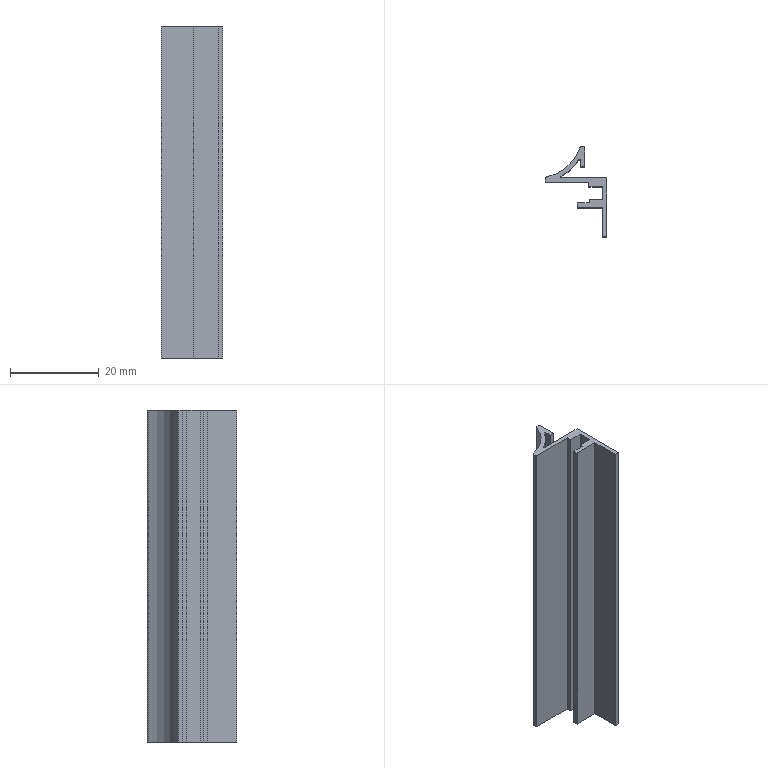Part | SolidWorks | features BaseBody 1, ICE 1, MoveFace 1 | 1 solid | 27 faces | box 14 x 20.3 x 75 mm | volume 3819 mm3 | plane 20 | cylinder 7 | commonest cylinder face diameters 0.387 x2 0.8 x2 0.4 x1 20 x1 22 x1
STEP:
#1=CARTESIAN_POINT('',(-5.304,-0.625,200.));
#2=VERTEX_POINT('',#1);
#3=CARTESIAN_POINT('',(-5.449,-0.8125,200.));
#4=VERTEX_POINT('',#3);
#5=CARTESIAN_POINT('',(-5.255,-0.8125,200.));
#6=DIRECTION('',(0.,0.,1.));
#7=DIRECTION('',(-1.,0.,0.));
#8=AXIS2_PLACEMENT_3D('',#5,#6,#7);
#9=CIRCLE('',#8,0.1937);
#10=EDGE_CURVE('',#2,#4,#9,.T.);
#11=ORIENTED_EDGE('',*,*,#10,.T.);
#12=CARTESIAN_POINT('',(-5.449,-0.8125,125.));
#13=VERTEX_POINT('',#12);
#14=CARTESIAN_POINT('',(-5.449,-0.8125,230.));
#15=DIRECTION('',(0.,0.,-1.));
#16=VECTOR('',#15,1000.);
#17=LINE('',#14,#16);
#18=EDGE_CURVE('',#4,#13,#17,.T.);
#19=ORIENTED_EDGE('',*,*,#18,.T.);
#20=CARTESIAN_POINT('',(-5.304,-0.625,125.));
#21=VERTEX_POINT('',#20);
#22=CARTESIAN_POINT('',(-5.255,-0.8125,125.));
#23=DIRECTION('',(0.,0.,-1.));
#24=DIRECTION('',(1.,0.,0.));
#25=AXIS2_PLACEMENT_3D('',#22,#23,#24);
#26=CIRCLE('',#25,0.1937);
#27=EDGE_CURVE('',#13,#21,#26,.T.);
#28=ORIENTED_EDGE('',*,*,#27,.T.);
#29=CARTESIAN_POINT('',(-5.304,-0.625,230.));
#30=DIRECTION('',(0.,0.,-1.));
#31=VECTOR('',#30,1000.);
#32=LINE('',#29,#31);
#33=EDGE_CURVE('',#2,#21,#32,.T.);
#34=ORIENTED_EDGE('',*,*,#33,.F.);
#35=EDGE_LOOP('',(#11,#19,#28,#34));
#36=FACE_OUTER_BOUND('',#35,.T.);
#37=CARTESIAN_POINT('',(-5.255,-0.8125,230.));
#38=DIRECTION('',(0.,0.,-1.));
#39=DIRECTION('',(-1.,0.,0.));
#40=AXIS2_PLACEMENT_3D('',#37,#38,#39);
#41=CYLINDRICAL_SURFACE('',#40,0.1937);
#42=ADVANCED_FACE('',(#36),#41,.F.);
#43=CARTESIAN_POINT('',(5.,-1.,125.));
#44=VERTEX_POINT('',#43);
#45=CARTESIAN_POINT('',(5.,-14.3,125.));
#46=VERTEX_POINT('',#45);
#47=CARTESIAN_POINT('',(5.,29.623,125.));
#48=DIRECTION('',(0.,-1.,0.));
#49=VECTOR('',#48,1000.);
#50=LINE('',#47,#49);
#51=EDGE_CURVE('',#44,#46,#50,.T.);
#52=ORIENTED_EDGE('',*,*,#51,.F.);
#53=CARTESIAN_POINT('',(5.,-1.,200.));
#54=VERTEX_POINT('',#53);
#55=CARTESIAN_POINT('',(5.,-1.,230.));
#56=DIRECTION('',(0.,0.,-1.));
#57=VECTOR('',#56,1000.);
#58=LINE('',#55,#57);
#59=EDGE_CURVE('',#54,#44,#58,.T.);
#60=ORIENTED_EDGE('',*,*,#59,.F.);
#61=CARTESIAN_POINT('',(5.,-14.3,200.));
#62=VERTEX_POINT('',#61);
#63=CARTESIAN_POINT('',(5.,-14.3,200.));
#64=DIRECTION('',(0.,1.,0.));
#65=VECTOR('',#64,1000.);
#66=LINE('',#63,#65);
#67=EDGE_CURVE('',#62,#54,#66,.T.);
#68=ORIENTED_EDGE('',*,*,#67,.F.);
#69=CARTESIAN_POINT('',(5.,-14.3,230.));
#70=DIRECTION('',(0.,0.,1.));
#71=VECTOR('',#70,1000.);
#72=LINE('',#69,#71);
#73=EDGE_CURVE('',#46,#62,#72,.T.);
#74=ORIENTED_EDGE('',*,*,#73,.F.);
#75=EDGE_LOOP('',(#52,#60,#68,#74));
#76=FACE_OUTER_BOUND('',#75,.T.);
#77=CARTESIAN_POINT('',(5.,-14.3,230.));
#78=DIRECTION('',(-1.,0.,0.));
#79=DIRECTION('',(0.,0.,1.));
#80=AXIS2_PLACEMENT_3D('',#77,#78,#79);
#81=PLANE('',#80);
#82=ADVANCED_FACE('',(#76),#81,.F.);
#83=CARTESIAN_POINT('',(-9.,-2.,125.));
#84=VERTEX_POINT('',#83);
#85=CARTESIAN_POINT('',(-9.,-2.,200.));
#86=VERTEX_POINT('',#85);
#87=CARTESIAN_POINT('',(-9.,-2.,230.));
#88=DIRECTION('',(0.,0.,1.));
#89=VECTOR('',#88,1000.);
#90=LINE('',#87,#89);
#91=EDGE_CURVE('',#84,#86,#90,.T.);
#92=ORIENTED_EDGE('',*,*,#91,.F.);
#93=CARTESIAN_POINT('',(0.9,-2.,125.));
#94=VERTEX_POINT('',#93);
#95=CARTESIAN_POINT('',(5.,-2.,125.));
#96=DIRECTION('',(-1.,0.,0.));
#97=VECTOR('',#96,1000.);
#98=LINE('',#95,#97);
#99=EDGE_CURVE('',#94,#84,#98,.T.);
#100=ORIENTED_EDGE('',*,*,#99,.F.);
#101=CARTESIAN_POINT('',(0.9,-2.,200.));
#102=VERTEX_POINT('',#101);
#103=CARTESIAN_POINT('',(0.9,-2.,230.));
#104=DIRECTION('',(0.,0.,-1.));
#105=VECTOR('',#104,1000.);
#106=LINE('',#103,#105);
#107=EDGE_CURVE('',#102,#94,#106,.T.);
#108=ORIENTED_EDGE('',*,*,#107,.F.);
#109=CARTESIAN_POINT('',(5.,-2.,200.));
#110=DIRECTION('',(1.,0.,0.));
#111=VECTOR('',#110,1000.);
#112=LINE('',#109,#111);
#113=EDGE_CURVE('',#86,#102,#112,.T.);
#114=ORIENTED_EDGE('',*,*,#113,.F.);
#115=EDGE_LOOP('',(#92,#100,#108,#114));
#116=FACE_OUTER_BOUND('',#115,.T.);
#117=CARTESIAN_POINT('',(-9.,-2.,230.));
#118=DIRECTION('',(0.,1.,0.));
#119=DIRECTION('',(0.,0.,1.));
#120=AXIS2_PLACEMENT_3D('',#117,#118,#119);
#121=PLANE('',#120);
#122=ADVANCED_FACE('',(#116),#121,.F.);
#123=CARTESIAN_POINT('',(4.,-6.,200.));
#124=VERTEX_POINT('',#123);
#125=CARTESIAN_POINT('',(4.,-3.,200.));
#126=VERTEX_POINT('',#125);
#127=CARTESIAN_POINT('',(4.,29.623,200.));
#128=DIRECTION('',(0.,1.,0.));
#129=VECTOR('',#128,1000.);
#130=LINE('',#127,#129);
#131=EDGE_CURVE('',#124,#126,#130,.T.);
#132=ORIENTED_EDGE('',*,*,#131,.F.);
#133=CARTESIAN_POINT('',(1.,-6.,200.));
#134=VERTEX_POINT('',#133);
#135=CARTESIAN_POINT('',(5.,-6.,200.));
#136=DIRECTION('',(1.,0.,0.));
#137=VECTOR('',#136,1000.);
#138=LINE('',#135,#137);
#139=EDGE_CURVE('',#134,#124,#138,.T.);
#140=ORIENTED_EDGE('',*,*,#139,.F.);
#141=CARTESIAN_POINT('',(1.,-6.7,200.));
#142=VERTEX_POINT('',#141);
#143=CARTESIAN_POINT('',(1.,-6.,200.));
#144=DIRECTION('',(0.,-1.,0.));
#145=VECTOR('',#144,1000.);
#146=LINE('',#143,#145);
#147=EDGE_CURVE('',#134,#142,#146,.T.);
#148=ORIENTED_EDGE('',*,*,#147,.T.);
#149=CARTESIAN_POINT('',(-1.7,-6.7,200.));
#150=VERTEX_POINT('',#149);
#151=CARTESIAN_POINT('',(5.,-6.7,200.));
#152=DIRECTION('',(1.,0.,0.));
#153=VECTOR('',#152,1000.);
#154=LINE('',#151,#153);
#155=EDGE_CURVE('',#150,#142,#154,.T.);
#156=ORIENTED_EDGE('',*,*,#155,.F.);
#157=CARTESIAN_POINT('',(-1.7,-7.7,200.));
#158=VERTEX_POINT('',#157);
#159=CARTESIAN_POINT('',(-1.7,-6.7,200.));
#160=DIRECTION('',(0.,-1.,0.));
#161=VECTOR('',#160,1000.);
#162=LINE('',#159,#161);
#163=EDGE_CURVE('',#150,#158,#162,.T.);
#164=ORIENTED_EDGE('',*,*,#163,.T.);
#165=CARTESIAN_POINT('',(4.,-7.7,200.));
#166=VERTEX_POINT('',#165);
#167=CARTESIAN_POINT('',(5.,-7.7,200.));
#168=DIRECTION('',(-1.,0.,0.));
#169=VECTOR('',#168,1000.);
#170=LINE('',#167,#169);
#171=EDGE_CURVE('',#166,#158,#170,.T.);
#172=ORIENTED_EDGE('',*,*,#171,.F.);
#173=CARTESIAN_POINT('',(4.,-14.3,200.));
#174=VERTEX_POINT('',#173);
#175=CARTESIAN_POINT('',(4.,29.623,200.));
#176=DIRECTION('',(0.,1.,0.));
#177=VECTOR('',#176,1000.);
#178=LINE('',#175,#177);
#179=EDGE_CURVE('',#174,#166,#178,.T.);
#180=ORIENTED_EDGE('',*,*,#179,.F.);
#181=CARTESIAN_POINT('',(5.,-14.3,200.));
#182=DIRECTION('',(-1.,0.,0.));
#183=VECTOR('',#182,1000.);
#184=LINE('',#181,#183);
#185=EDGE_CURVE('',#62,#174,#184,.T.);
#186=ORIENTED_EDGE('',*,*,#185,.F.);
#187=ORIENTED_EDGE('',*,*,#67,.T.);
#188=CARTESIAN_POINT('',(-5.207,-1.,200.));
#189=VERTEX_POINT('',#188);
#190=CARTESIAN_POINT('',(5.,-1.,200.));
#191=DIRECTION('',(1.,0.,0.));
#192=VECTOR('',#191,1000.);
#193=LINE('',#190,#192);
#194=EDGE_CURVE('',#189,#54,#193,.T.);
#195=ORIENTED_EDGE('',*,*,#194,.F.);
#196=CARTESIAN_POINT('',(-5.255,-0.8125,200.));
#197=DIRECTION('',(0.,0.,1.));
#198=DIRECTION('',(-1.,0.,0.));
#199=AXIS2_PLACEMENT_3D('',#196,#197,#198);
#200=CIRCLE('',#199,0.1937);
#201=EDGE_CURVE('',#4,#189,#200,.T.);
#202=ORIENTED_EDGE('',*,*,#201,.F.);
#203=ORIENTED_EDGE('',*,*,#10,.F.);
#204=CARTESIAN_POINT('',(-1.368,3.063,200.));
#205=VERTEX_POINT('',#204);
#206=CARTESIAN_POINT('',(-10.628,9.,200.));
#207=DIRECTION('',(0.,0.,1.));
#208=DIRECTION('',(-1.,0.,0.));
#209=AXIS2_PLACEMENT_3D('',#206,#207,#208);
#210=CIRCLE('',#209,11.);
#211=EDGE_CURVE('',#2,#205,#210,.T.);
#212=ORIENTED_EDGE('',*,*,#211,.T.);
#213=CARTESIAN_POINT('',(-1.,2.955,200.));
#214=VERTEX_POINT('',#213);
#215=CARTESIAN_POINT('',(-1.2,2.955,200.));
#216=DIRECTION('',(0.,0.,1.));
#217=DIRECTION('',(-1.,0.,0.));
#218=AXIS2_PLACEMENT_3D('',#215,#216,#217);
#219=CIRCLE('',#218,0.2);
#220=EDGE_CURVE('',#214,#205,#219,.T.);
#221=ORIENTED_EDGE('',*,*,#220,.F.);
#222=CARTESIAN_POINT('',(-1.,1.5,200.));
#223=VERTEX_POINT('',#222);
#224=CARTESIAN_POINT('',(-1.,2.955,200.));
#225=DIRECTION('',(0.,1.,0.));
#226=VECTOR('',#225,1000.);
#227=LINE('',#224,#226);
#228=EDGE_CURVE('',#223,#214,#227,.T.);
#229=ORIENTED_EDGE('',*,*,#228,.F.);
#230=CARTESIAN_POINT('',(0.,1.5,200.));
#231=VERTEX_POINT('',#230);
#232=CARTESIAN_POINT('',(-1.,1.5,200.));
#233=DIRECTION('',(-1.,0.,0.));
#234=VECTOR('',#233,1000.);
#235=LINE('',#232,#234);
#236=EDGE_CURVE('',#231,#223,#235,.T.);
#237=ORIENTED_EDGE('',*,*,#236,.F.);
#238=CARTESIAN_POINT('',(0.,6.,200.));
#239=VERTEX_POINT('',#238);
#240=CARTESIAN_POINT('',(0.,1.5,200.));
#241=DIRECTION('',(0.,-1.,0.));
#242=VECTOR('',#241,1000.);
#243=LINE('',#240,#242);
#244=EDGE_CURVE('',#239,#231,#243,.T.);
#245=ORIENTED_EDGE('',*,*,#244,.F.);
#246=CARTESIAN_POINT('',(-0.8,6.,200.));
#247=VERTEX_POINT('',#246);
#248=CARTESIAN_POINT('',(0.,6.,200.));
#249=DIRECTION('',(1.,0.,0.));
#250=VECTOR('',#249,1000.);
#251=LINE('',#248,#250);
#252=EDGE_CURVE('',#247,#239,#251,.T.);
#253=ORIENTED_EDGE('',*,*,#252,.F.);
#254=CARTESIAN_POINT('',(-1.178,5.731,200.));
#255=VERTEX_POINT('',#254);
#256=CARTESIAN_POINT('',(-0.8,5.6,200.));
#257=DIRECTION('',(0.,0.,1.));
#258=DIRECTION('',(-1.,0.,0.));
#259=AXIS2_PLACEMENT_3D('',#256,#257,#258);
#260=CIRCLE('',#259,0.4);
#261=EDGE_CURVE('',#247,#255,#260,.T.);
#262=ORIENTED_EDGE('',*,*,#261,.T.);
#263=CARTESIAN_POINT('',(-8.678,-0.8077,200.));
#264=VERTEX_POINT('',#263);
#265=CARTESIAN_POINT('',(-10.628,9.,200.));
#266=DIRECTION('',(0.,0.,1.));
#267=DIRECTION('',(-1.,0.,0.));
#268=AXIS2_PLACEMENT_3D('',#265,#266,#267);
#269=CIRCLE('',#268,10.);
#270=EDGE_CURVE('',#264,#255,#269,.T.);
#271=ORIENTED_EDGE('',*,*,#270,.F.);
#272=CARTESIAN_POINT('',(-9.,-1.2,200.));
#273=VERTEX_POINT('',#272);
#274=CARTESIAN_POINT('',(-8.6,-1.2,200.));
#275=DIRECTION('',(0.,0.,1.));
#276=DIRECTION('',(-1.,0.,0.));
#277=AXIS2_PLACEMENT_3D('',#274,#275,#276);
#278=CIRCLE('',#277,0.4);
#279=EDGE_CURVE('',#264,#273,#278,.T.);
#280=ORIENTED_EDGE('',*,*,#279,.T.);
#281=CARTESIAN_POINT('',(-9.,8.,200.));
#282=DIRECTION('',(0.,-1.,0.));
#283=VECTOR('',#282,1000.);
#284=LINE('',#281,#283);
#285=EDGE_CURVE('',#273,#86,#284,.T.);
#286=ORIENTED_EDGE('',*,*,#285,.T.);
#287=ORIENTED_EDGE('',*,*,#113,.T.);
#288=CARTESIAN_POINT('',(0.9,-3.,200.));
#289=VERTEX_POINT('',#288);
#290=CARTESIAN_POINT('',(0.9,29.623,200.));
#291=DIRECTION('',(0.,1.,0.));
#292=VECTOR('',#291,1000.);
#293=LINE('',#290,#292);
#294=EDGE_CURVE('',#289,#102,#293,.T.);
#295=ORIENTED_EDGE('',*,*,#294,.F.);
#296=CARTESIAN_POINT('',(5.,-3.,200.));
#297=DIRECTION('',(-1.,0.,0.));
#298=VECTOR('',#297,1000.);
#299=LINE('',#296,#298);
#300=EDGE_CURVE('',#126,#289,#299,.T.);
#301=ORIENTED_EDGE('',*,*,#300,.F.);
#302=EDGE_LOOP('',(#132,#140,#148,#156,#164,#172,#180,#186,#187,#195,#202,#203,#212,#221,#229,#237,#245,#253,#262,#271,#280,#286,#287,#295,#301));
#303=FACE_OUTER_BOUND('',#302,.T.);
#304=CARTESIAN_POINT('',(5.,29.623,200.));
#305=DIRECTION('',(0.,0.,-1.));
#306=DIRECTION('',(-1.,0.,0.));
#307=AXIS2_PLACEMENT_3D('',#304,#305,#306);
#308=PLANE('',#307);
#309=ADVANCED_FACE('',(#303),#308,.F.);
#310=ORIENTED_EDGE('',*,*,#185,.T.);
#311=CARTESIAN_POINT('',(4.,-14.3,125.));
#312=VERTEX_POINT('',#311);
#313=CARTESIAN_POINT('',(4.,-14.3,230.));
#314=DIRECTION('',(0.,0.,1.));
#315=VECTOR('',#314,1000.);
#316=LINE('',#313,#315);
#317=EDGE_CURVE('',#312,#174,#316,.T.);
#318=ORIENTED_EDGE('',*,*,#317,.F.);
#319=CARTESIAN_POINT('',(5.,-14.3,125.));
#320=DIRECTION('',(-1.,0.,0.));
#321=VECTOR('',#320,1000.);
#322=LINE('',#319,#321);
#323=EDGE_CURVE('',#46,#312,#322,.T.);
#324=ORIENTED_EDGE('',*,*,#323,.F.);
#325=ORIENTED_EDGE('',*,*,#73,.T.);
#326=EDGE_LOOP('',(#310,#318,#324,#325));
#327=FACE_OUTER_BOUND('',#326,.T.);
#328=CARTESIAN_POINT('',(4.,-14.3,230.));
#329=DIRECTION('',(0.,1.,0.));
#330=DIRECTION('',(0.,0.,1.));
#331=AXIS2_PLACEMENT_3D('',#328,#329,#330);
#332=PLANE('',#331);
#333=ADVANCED_FACE('',(#327),#332,.F.);
#334=ORIENTED_EDGE('',*,*,#51,.T.);
#335=ORIENTED_EDGE('',*,*,#323,.T.);
#336=CARTESIAN_POINT('',(4.,-7.7,125.));
#337=VERTEX_POINT('',#336);
#338=CARTESIAN_POINT('',(4.,-7.7,125.));
#339=DIRECTION('',(0.,-1.,0.));
#340=VECTOR('',#339,1000.);
#341=LINE('',#338,#340);
#342=EDGE_CURVE('',#337,#312,#341,.T.);
#343=ORIENTED_EDGE('',*,*,#342,.F.);
#344=CARTESIAN_POINT('',(-1.7,-7.7,125.));
#345=VERTEX_POINT('',#344);
#346=CARTESIAN_POINT('',(-1.7,-7.7,125.));
#347=DIRECTION('',(1.,0.,0.));
#348=VECTOR('',#347,1000.);
#349=LINE('',#346,#348);
#350=EDGE_CURVE('',#345,#337,#349,.T.);
#351=ORIENTED_EDGE('',*,*,#350,.F.);
#352=CARTESIAN_POINT('',(-1.7,-6.7,125.));
#353=VERTEX_POINT('',#352);
#354=CARTESIAN_POINT('',(-1.7,29.623,125.));
#355=DIRECTION('',(0.,1.,0.));
#356=VECTOR('',#355,1000.);
#357=LINE('',#354,#356);
#358=EDGE_CURVE('',#345,#353,#357,.T.);
#359=ORIENTED_EDGE('',*,*,#358,.T.);
#360=CARTESIAN_POINT('',(1.,-6.7,125.));
#361=VERTEX_POINT('',#360);
#362=CARTESIAN_POINT('',(1.,-6.7,125.));
#363=DIRECTION('',(-1.,0.,0.));
#364=VECTOR('',#363,1000.);
#365=LINE('',#362,#364);
#366=EDGE_CURVE('',#361,#353,#365,.T.);
#367=ORIENTED_EDGE('',*,*,#366,.F.);
#368=CARTESIAN_POINT('',(1.,-6.,125.));
#369=VERTEX_POINT('',#368);
#370=CARTESIAN_POINT('',(1.,29.623,125.));
#371=DIRECTION('',(0.,1.,0.));
#372=VECTOR('',#371,1000.);
#373=LINE('',#370,#372);
#374=EDGE_CURVE('',#361,#369,#373,.T.);
#375=ORIENTED_EDGE('',*,*,#374,.T.);
#376=CARTESIAN_POINT('',(4.,-6.,125.));
#377=VERTEX_POINT('',#376);
#378=CARTESIAN_POINT('',(4.,-6.,125.));
#379=DIRECTION('',(-1.,0.,0.));
#380=VECTOR('',#379,1000.);
#381=LINE('',#378,#380);
#382=EDGE_CURVE('',#377,#369,#381,.T.);
#383=ORIENTED_EDGE('',*,*,#382,.F.);
#384=CARTESIAN_POINT('',(4.,-3.,125.));
#385=VERTEX_POINT('',#384);
#386=CARTESIAN_POINT('',(4.,-3.,125.));
#387=DIRECTION('',(0.,-1.,0.));
#388=VECTOR('',#387,1000.);
#389=LINE('',#386,#388);
#390=EDGE_CURVE('',#385,#377,#389,.T.);
#391=ORIENTED_EDGE('',*,*,#390,.F.);
#392=CARTESIAN_POINT('',(0.9,-3.,125.));
#393=VERTEX_POINT('',#392);
#394=CARTESIAN_POINT('',(0.9,-3.,125.));
#395=DIRECTION('',(1.,0.,0.));
#396=VECTOR('',#395,1000.);
#397=LINE('',#394,#396);
#398=EDGE_CURVE('',#393,#385,#397,.T.);
#399=ORIENTED_EDGE('',*,*,#398,.F.);
#400=CARTESIAN_POINT('',(0.9,-2.,125.));
#401=DIRECTION('',(0.,-1.,0.));
#402=VECTOR('',#401,1000.);
#403=LINE('',#400,#402);
#404=EDGE_CURVE('',#94,#393,#403,.T.);
#405=ORIENTED_EDGE('',*,*,#404,.F.);
#406=ORIENTED_EDGE('',*,*,#99,.T.);
#407=CARTESIAN_POINT('',(-9.,-1.2,125.));
#408=VERTEX_POINT('',#407);
#409=CARTESIAN_POINT('',(-9.,-1.2,125.));
#410=DIRECTION('',(0.,-1.,0.));
#411=VECTOR('',#410,1000.);
#412=LINE('',#409,#411);
#413=EDGE_CURVE('',#408,#84,#412,.T.);
#414=ORIENTED_EDGE('',*,*,#413,.F.);
#415=CARTESIAN_POINT('',(-8.678,-0.8077,125.));
#416=VERTEX_POINT('',#415);
#417=CARTESIAN_POINT('',(-8.6,-1.2,125.));
#418=DIRECTION('',(0.,0.,-1.));
#419=DIRECTION('',(1.,0.,0.));
#420=AXIS2_PLACEMENT_3D('',#417,#418,#419);
#421=CIRCLE('',#420,0.4);
#422=EDGE_CURVE('',#408,#416,#421,.T.);
#423=ORIENTED_EDGE('',*,*,#422,.T.);
#424=CARTESIAN_POINT('',(-1.178,5.731,125.));
#425=VERTEX_POINT('',#424);
#426=CARTESIAN_POINT('',(-10.628,9.,125.));
#427=DIRECTION('',(0.,0.,-1.));
#428=DIRECTION('',(1.,0.,0.));
#429=AXIS2_PLACEMENT_3D('',#426,#427,#428);
#430=CIRCLE('',#429,10.);
#431=EDGE_CURVE('',#425,#416,#430,.T.);
#432=ORIENTED_EDGE('',*,*,#431,.F.);
#433=CARTESIAN_POINT('',(-0.8,6.,125.));
#434=VERTEX_POINT('',#433);
#435=CARTESIAN_POINT('',(-0.8,5.6,125.));
#436=DIRECTION('',(0.,0.,-1.));
#437=DIRECTION('',(1.,0.,0.));
#438=AXIS2_PLACEMENT_3D('',#435,#436,#437);
#439=CIRCLE('',#438,0.4);
#440=EDGE_CURVE('',#425,#434,#439,.T.);
#441=ORIENTED_EDGE('',*,*,#440,.T.);
#442=CARTESIAN_POINT('',(0.,6.,125.));
#443=VERTEX_POINT('',#442);
#444=CARTESIAN_POINT('',(0.,6.,125.));
#445=DIRECTION('',(-1.,0.,0.));
#446=VECTOR('',#445,1000.);
#447=LINE('',#444,#446);
#448=EDGE_CURVE('',#443,#434,#447,.T.);
#449=ORIENTED_EDGE('',*,*,#448,.F.);
#450=CARTESIAN_POINT('',(0.,1.5,125.));
#451=VERTEX_POINT('',#450);
#452=CARTESIAN_POINT('',(0.,1.5,125.));
#453=DIRECTION('',(0.,1.,0.));
#454=VECTOR('',#453,1000.);
#455=LINE('',#452,#454);
#456=EDGE_CURVE('',#451,#443,#455,.T.);
#457=ORIENTED_EDGE('',*,*,#456,.F.);
#458=CARTESIAN_POINT('',(-1.,1.5,125.));
#459=VERTEX_POINT('',#458);
#460=CARTESIAN_POINT('',(-1.,1.5,125.));
#461=DIRECTION('',(1.,0.,0.));
#462=VECTOR('',#461,1000.);
#463=LINE('',#460,#462);
#464=EDGE_CURVE('',#459,#451,#463,.T.);
#465=ORIENTED_EDGE('',*,*,#464,.F.);
#466=CARTESIAN_POINT('',(-1.,2.955,125.));
#467=VERTEX_POINT('',#466);
#468=CARTESIAN_POINT('',(-1.,2.955,125.));
#469=DIRECTION('',(0.,-1.,0.));
#470=VECTOR('',#469,1000.);
#471=LINE('',#468,#470);
#472=EDGE_CURVE('',#467,#459,#471,.T.);
#473=ORIENTED_EDGE('',*,*,#472,.F.);
#474=CARTESIAN_POINT('',(-1.368,3.063,125.));
#475=VERTEX_POINT('',#474);
#476=CARTESIAN_POINT('',(-1.2,2.955,125.));
#477=DIRECTION('',(0.,0.,-1.));
#478=DIRECTION('',(1.,0.,0.));
#479=AXIS2_PLACEMENT_3D('',#476,#477,#478);
#480=CIRCLE('',#479,0.2);
#481=EDGE_CURVE('',#475,#467,#480,.T.);
#482=ORIENTED_EDGE('',*,*,#481,.F.);
#483=CARTESIAN_POINT('',(-10.628,9.,125.));
#484=DIRECTION('',(0.,0.,-1.));
#485=DIRECTION('',(1.,0.,0.));
#486=AXIS2_PLACEMENT_3D('',#483,#484,#485);
#487=CIRCLE('',#486,11.);
#488=EDGE_CURVE('',#475,#21,#487,.T.);
#489=ORIENTED_EDGE('',*,*,#488,.T.);
#490=ORIENTED_EDGE('',*,*,#27,.F.);
#491=CARTESIAN_POINT('',(-5.207,-1.,125.));
#492=VERTEX_POINT('',#491);
#493=CARTESIAN_POINT('',(-5.255,-0.8125,125.));
#494=DIRECTION('',(0.,0.,-1.));
#495=DIRECTION('',(1.,0.,0.));
#496=AXIS2_PLACEMENT_3D('',#493,#494,#495);
#497=CIRCLE('',#496,0.1937);
#498=EDGE_CURVE('',#492,#13,#497,.T.);
#499=ORIENTED_EDGE('',*,*,#498,.F.);
#500=CARTESIAN_POINT('',(5.,-1.,125.));
#501=DIRECTION('',(-1.,0.,0.));
#502=VECTOR('',#501,1000.);
#503=LINE('',#500,#502);
#504=EDGE_CURVE('',#44,#492,#503,.T.);
#505=ORIENTED_EDGE('',*,*,#504,.F.);
#506=EDGE_LOOP('',(#334,#335,#343,#351,#359,#367,#375,#383,#391,#399,#405,#406,#414,#423,#432,#441,#449,#457,#465,#473,#482,#489,#490,#499,#505));
#507=FACE_OUTER_BOUND('',#506,.T.);
#508=CARTESIAN_POINT('',(5.,29.623,125.));
#509=DIRECTION('',(0.,0.,1.));
#510=DIRECTION('',(1.,0.,0.));
#511=AXIS2_PLACEMENT_3D('',#508,#509,#510);
#512=PLANE('',#511);
#513=ADVANCED_FACE('',(#507),#512,.F.);
#514=ORIENTED_EDGE('',*,*,#59,.T.);
#515=ORIENTED_EDGE('',*,*,#504,.T.);
#516=CARTESIAN_POINT('',(-5.207,-1.,230.));
#517=DIRECTION('',(0.,0.,-1.));
#518=VECTOR('',#517,1000.);
#519=LINE('',#516,#518);
#520=EDGE_CURVE('',#189,#492,#519,.T.);
#521=ORIENTED_EDGE('',*,*,#520,.F.);
#522=ORIENTED_EDGE('',*,*,#194,.T.);
#523=EDGE_LOOP('',(#514,#515,#521,#522));
#524=FACE_OUTER_BOUND('',#523,.T.);
#525=CARTESIAN_POINT('',(5.,-1.,230.));
#526=DIRECTION('',(0.,-1.,0.));
#527=DIRECTION('',(0.,0.,-1.));
#528=AXIS2_PLACEMENT_3D('',#525,#526,#527);
#529=PLANE('',#528);
#530=ADVANCED_FACE('',(#524),#529,.F.);
#531=CARTESIAN_POINT('',(-9.,-1.2,230.));
#532=DIRECTION('',(0.,0.,1.));
#533=VECTOR('',#532,1000.);
#534=LINE('',#531,#533);
#535=EDGE_CURVE('',#408,#273,#534,.T.);
#536=ORIENTED_EDGE('',*,*,#535,.F.);
#537=ORIENTED_EDGE('',*,*,#413,.T.);
#538=ORIENTED_EDGE('',*,*,#91,.T.);
#539=ORIENTED_EDGE('',*,*,#285,.F.);
#540=EDGE_LOOP('',(#536,#537,#538,#539));
#541=FACE_OUTER_BOUND('',#540,.T.);
#542=CARTESIAN_POINT('',(-9.,-1.2,230.));
#543=DIRECTION('',(1.,0.,0.));
#544=DIRECTION('',(0.,0.,-1.));
#545=AXIS2_PLACEMENT_3D('',#542,#543,#544);
#546=PLANE('',#545);
#547=ADVANCED_FACE('',(#541),#546,.F.);
#548=ORIENTED_EDGE('',*,*,#294,.T.);
#549=ORIENTED_EDGE('',*,*,#107,.T.);
#550=ORIENTED_EDGE('',*,*,#404,.T.);
#551=CARTESIAN_POINT('',(0.9,-3.,230.));
#552=DIRECTION('',(0.,0.,-1.));
#553=VECTOR('',#552,1000.);
#554=LINE('',#551,#553);
#555=EDGE_CURVE('',#289,#393,#554,.T.);
#556=ORIENTED_EDGE('',*,*,#555,.F.);
#557=EDGE_LOOP('',(#548,#549,#550,#556));
#558=FACE_OUTER_BOUND('',#557,.T.);
#559=CARTESIAN_POINT('',(0.9,-2.,230.));
#560=DIRECTION('',(1.,0.,0.));
#561=DIRECTION('',(0.,0.,-1.));
#562=AXIS2_PLACEMENT_3D('',#559,#560,#561);
#563=PLANE('',#562);
#564=ADVANCED_FACE('',(#558),#563,.F.);
#565=ORIENTED_EDGE('',*,*,#300,.T.);
#566=ORIENTED_EDGE('',*,*,#555,.T.);
#567=ORIENTED_EDGE('',*,*,#398,.T.);
#568=CARTESIAN_POINT('',(4.,-3.,230.));
#569=DIRECTION('',(0.,0.,-1.));
#570=VECTOR('',#569,1000.);
#571=LINE('',#568,#570);
#572=EDGE_CURVE('',#126,#385,#571,.T.);
#573=ORIENTED_EDGE('',*,*,#572,.F.);
#574=EDGE_LOOP('',(#565,#566,#567,#573));
#575=FACE_OUTER_BOUND('',#574,.T.);
#576=CARTESIAN_POINT('',(0.9,-3.,230.));
#577=DIRECTION('',(0.,1.,0.));
#578=DIRECTION('',(0.,0.,1.));
#579=AXIS2_PLACEMENT_3D('',#576,#577,#578);
#580=PLANE('',#579);
#581=ADVANCED_FACE('',(#575),#580,.F.);
#582=ORIENTED_EDGE('',*,*,#131,.T.);
#583=ORIENTED_EDGE('',*,*,#572,.T.);
#584=ORIENTED_EDGE('',*,*,#390,.T.);
#585=CARTESIAN_POINT('',(4.,-6.,230.));
#586=DIRECTION('',(0.,0.,-1.));
#587=VECTOR('',#586,1000.);
#588=LINE('',#585,#587);
#589=EDGE_CURVE('',#124,#377,#588,.T.);
#590=ORIENTED_EDGE('',*,*,#589,.F.);
#591=EDGE_LOOP('',(#582,#583,#584,#590));
#592=FACE_OUTER_BOUND('',#591,.T.);
#593=CARTESIAN_POINT('',(4.,-3.,230.));
#594=DIRECTION('',(1.,0.,0.));
#595=DIRECTION('',(0.,0.,-1.));
#596=AXIS2_PLACEMENT_3D('',#593,#594,#595);
#597=PLANE('',#596);
#598=ADVANCED_FACE('',(#592),#597,.F.);
#599=ORIENTED_EDGE('',*,*,#139,.T.);
#600=ORIENTED_EDGE('',*,*,#589,.T.);
#601=ORIENTED_EDGE('',*,*,#382,.T.);
#602=CARTESIAN_POINT('',(1.,-6.,230.));
#603=DIRECTION('',(0.,0.,-1.));
#604=VECTOR('',#603,1000.);
#605=LINE('',#602,#604);
#606=EDGE_CURVE('',#134,#369,#605,.T.);
#607=ORIENTED_EDGE('',*,*,#606,.F.);
#608=EDGE_LOOP('',(#599,#600,#601,#607));
#609=FACE_OUTER_BOUND('',#608,.T.);
#610=CARTESIAN_POINT('',(4.,-6.,230.));
#611=DIRECTION('',(0.,-1.,0.));
#612=DIRECTION('',(0.,0.,-1.));
#613=AXIS2_PLACEMENT_3D('',#610,#611,#612);
#614=PLANE('',#613);
#615=ADVANCED_FACE('',(#609),#614,.F.);
#616=ORIENTED_EDGE('',*,*,#155,.T.);
#617=CARTESIAN_POINT('',(1.,-6.7,230.));
#618=DIRECTION('',(0.,0.,1.));
#619=VECTOR('',#618,1000.);
#620=LINE('',#617,#619);
#621=EDGE_CURVE('',#361,#142,#620,.T.);
#622=ORIENTED_EDGE('',*,*,#621,.F.);
#623=ORIENTED_EDGE('',*,*,#366,.T.);
#624=CARTESIAN_POINT('',(-1.7,-6.7,230.));
#625=DIRECTION('',(0.,0.,-1.));
#626=VECTOR('',#625,1000.);
#627=LINE('',#624,#626);
#628=EDGE_CURVE('',#150,#353,#627,.T.);
#629=ORIENTED_EDGE('',*,*,#628,.F.);
#630=EDGE_LOOP('',(#616,#622,#623,#629));
#631=FACE_OUTER_BOUND('',#630,.T.);
#632=CARTESIAN_POINT('',(1.,-6.7,230.));
#633=DIRECTION('',(0.,-1.,0.));
#634=DIRECTION('',(0.,0.,-1.));
#635=AXIS2_PLACEMENT_3D('',#632,#633,#634);
#636=PLANE('',#635);
#637=ADVANCED_FACE('',(#631),#636,.F.);
#638=ORIENTED_EDGE('',*,*,#171,.T.);
#639=CARTESIAN_POINT('',(-1.7,-7.7,230.));
#640=DIRECTION('',(0.,0.,1.));
#641=VECTOR('',#640,1000.);
#642=LINE('',#639,#641);
#643=EDGE_CURVE('',#345,#158,#642,.T.);
#644=ORIENTED_EDGE('',*,*,#643,.F.);
#645=ORIENTED_EDGE('',*,*,#350,.T.);
#646=CARTESIAN_POINT('',(4.,-7.7,230.));
#647=DIRECTION('',(0.,0.,-1.));
#648=VECTOR('',#647,1000.);
#649=LINE('',#646,#648);
#650=EDGE_CURVE('',#166,#337,#649,.T.);
#651=ORIENTED_EDGE('',*,*,#650,.F.);
#652=EDGE_LOOP('',(#638,#644,#645,#651));
#653=FACE_OUTER_BOUND('',#652,.T.);
#654=CARTESIAN_POINT('',(-1.7,-7.7,230.));
#655=DIRECTION('',(0.,1.,0.));
#656=DIRECTION('',(0.,0.,1.));
#657=AXIS2_PLACEMENT_3D('',#654,#655,#656);
#658=PLANE('',#657);
#659=ADVANCED_FACE('',(#653),#658,.F.);
#660=ORIENTED_EDGE('',*,*,#179,.T.);
#661=ORIENTED_EDGE('',*,*,#650,.T.);
#662=ORIENTED_EDGE('',*,*,#342,.T.);
#663=ORIENTED_EDGE('',*,*,#317,.T.);
#664=EDGE_LOOP('',(#660,#661,#662,#663));
#665=FACE_OUTER_BOUND('',#664,.T.);
#666=CARTESIAN_POINT('',(4.,-7.7,230.));
#667=DIRECTION('',(1.,0.,0.));
#668=DIRECTION('',(0.,0.,-1.));
#669=AXIS2_PLACEMENT_3D('',#666,#667,#668);
#670=PLANE('',#669);
#671=ADVANCED_FACE('',(#665),#670,.F.);
#672=ORIENTED_EDGE('',*,*,#18,.F.);
#673=ORIENTED_EDGE('',*,*,#201,.T.);
#674=ORIENTED_EDGE('',*,*,#520,.T.);
#675=ORIENTED_EDGE('',*,*,#498,.T.);
#676=EDGE_LOOP('',(#672,#673,#674,#675));
#677=FACE_OUTER_BOUND('',#676,.T.);
#678=CARTESIAN_POINT('',(-5.255,-0.8125,230.));
#679=DIRECTION('',(0.,0.,-1.));
#680=DIRECTION('',(-1.,0.,0.));
#681=AXIS2_PLACEMENT_3D('',#678,#679,#680);
#682=CYLINDRICAL_SURFACE('',#681,0.1937);
#683=ADVANCED_FACE('',(#677),#682,.F.);
#684=CARTESIAN_POINT('',(-1.,2.955,230.));
#685=DIRECTION('',(0.,0.,1.));
#686=VECTOR('',#685,1000.);
#687=LINE('',#684,#686);
#688=EDGE_CURVE('',#467,#214,#687,.T.);
#689=ORIENTED_EDGE('',*,*,#688,.F.);
#690=ORIENTED_EDGE('',*,*,#472,.T.);
#691=CARTESIAN_POINT('',(-1.,1.5,230.));
#692=DIRECTION('',(0.,0.,-1.));
#693=VECTOR('',#692,1000.);
#694=LINE('',#691,#693);
#695=EDGE_CURVE('',#223,#459,#694,.T.);
#696=ORIENTED_EDGE('',*,*,#695,.F.);
#697=ORIENTED_EDGE('',*,*,#228,.T.);
#698=EDGE_LOOP('',(#689,#690,#696,#697));
#699=FACE_OUTER_BOUND('',#698,.T.);
#700=CARTESIAN_POINT('',(-1.,2.955,230.));
#701=DIRECTION('',(1.,0.,0.));
#702=DIRECTION('',(0.,0.,-1.));
#703=AXIS2_PLACEMENT_3D('',#700,#701,#702);
#704=PLANE('',#703);
#705=ADVANCED_FACE('',(#699),#704,.F.);
#706=ORIENTED_EDGE('',*,*,#488,.F.);
#707=CARTESIAN_POINT('',(-1.368,3.063,230.));
#708=DIRECTION('',(0.,0.,1.));
#709=VECTOR('',#708,1000.);
#710=LINE('',#707,#709);
#711=EDGE_CURVE('',#475,#205,#710,.T.);
#712=ORIENTED_EDGE('',*,*,#711,.T.);
#713=ORIENTED_EDGE('',*,*,#211,.F.);
#714=ORIENTED_EDGE('',*,*,#33,.T.);
#715=EDGE_LOOP('',(#706,#712,#713,#714));
#716=FACE_OUTER_BOUND('',#715,.T.);
#717=CARTESIAN_POINT('',(-10.628,9.,230.));
#718=DIRECTION('',(0.,0.,-1.));
#719=DIRECTION('',(-1.,0.,0.));
#720=AXIS2_PLACEMENT_3D('',#717,#718,#719);
#721=CYLINDRICAL_SURFACE('',#720,11.);
#722=ADVANCED_FACE('',(#716),#721,.T.);
#723=CARTESIAN_POINT('',(-1.178,5.731,230.));
#724=DIRECTION('',(0.,0.,1.));
#725=VECTOR('',#724,1000.);
#726=LINE('',#723,#725);
#727=EDGE_CURVE('',#425,#255,#726,.T.);
#728=ORIENTED_EDGE('',*,*,#727,.F.);
#729=ORIENTED_EDGE('',*,*,#431,.T.);
#730=CARTESIAN_POINT('',(-8.678,-0.8077,230.));
#731=DIRECTION('',(0.,0.,-1.));
#732=VECTOR('',#731,1000.);
#733=LINE('',#730,#732);
#734=EDGE_CURVE('',#264,#416,#733,.T.);
#735=ORIENTED_EDGE('',*,*,#734,.F.);
#736=ORIENTED_EDGE('',*,*,#270,.T.);
#737=EDGE_LOOP('',(#728,#729,#735,#736));
#738=FACE_OUTER_BOUND('',#737,.T.);
#739=CARTESIAN_POINT('',(-10.628,9.,230.));
#740=DIRECTION('',(0.,0.,-1.));
#741=DIRECTION('',(-1.,0.,0.));
#742=AXIS2_PLACEMENT_3D('',#739,#740,#741);
#743=CYLINDRICAL_SURFACE('',#742,10.);
#744=ADVANCED_FACE('',(#738),#743,.F.);
#745=CARTESIAN_POINT('',(0.,1.5,230.));
#746=DIRECTION('',(0.,0.,1.));
#747=VECTOR('',#746,1000.);
#748=LINE('',#745,#747);
#749=EDGE_CURVE('',#451,#231,#748,.T.);
#750=ORIENTED_EDGE('',*,*,#749,.F.);
#751=ORIENTED_EDGE('',*,*,#456,.T.);
#752=CARTESIAN_POINT('',(0.,6.,230.));
#753=DIRECTION('',(0.,0.,-1.));
#754=VECTOR('',#753,1000.);
#755=LINE('',#752,#754);
#756=EDGE_CURVE('',#239,#443,#755,.T.);
#757=ORIENTED_EDGE('',*,*,#756,.F.);
#758=ORIENTED_EDGE('',*,*,#244,.T.);
#759=EDGE_LOOP('',(#750,#751,#757,#758));
#760=FACE_OUTER_BOUND('',#759,.T.);
#761=CARTESIAN_POINT('',(0.,1.5,230.));
#762=DIRECTION('',(-1.,0.,0.));
#763=DIRECTION('',(0.,0.,1.));
#764=AXIS2_PLACEMENT_3D('',#761,#762,#763);
#765=PLANE('',#764);
#766=ADVANCED_FACE('',(#760),#765,.F.);
#767=ORIENTED_EDGE('',*,*,#422,.F.);
#768=ORIENTED_EDGE('',*,*,#535,.T.);
#769=ORIENTED_EDGE('',*,*,#279,.F.);
#770=ORIENTED_EDGE('',*,*,#734,.T.);
#771=EDGE_LOOP('',(#767,#768,#769,#770));
#772=FACE_OUTER_BOUND('',#771,.T.);
#773=CARTESIAN_POINT('',(-8.6,-1.2,230.));
#774=DIRECTION('',(0.,0.,-1.));
#775=DIRECTION('',(-1.,0.,0.));
#776=AXIS2_PLACEMENT_3D('',#773,#774,#775);
#777=CYLINDRICAL_SURFACE('',#776,0.4);
#778=ADVANCED_FACE('',(#772),#777,.T.);
#779=ORIENTED_EDGE('',*,*,#147,.F.);
#780=ORIENTED_EDGE('',*,*,#606,.T.);
#781=ORIENTED_EDGE('',*,*,#374,.F.);
#782=ORIENTED_EDGE('',*,*,#621,.T.);
#783=EDGE_LOOP('',(#779,#780,#781,#782));
#784=FACE_OUTER_BOUND('',#783,.T.);
#785=CARTESIAN_POINT('',(1.,-6.,230.));
#786=DIRECTION('',(1.,0.,0.));
#787=DIRECTION('',(0.,0.,-1.));
#788=AXIS2_PLACEMENT_3D('',#785,#786,#787);
#789=PLANE('',#788);
#790=ADVANCED_FACE('',(#784),#789,.F.);
#791=ORIENTED_EDGE('',*,*,#163,.F.);
#792=ORIENTED_EDGE('',*,*,#628,.T.);
#793=ORIENTED_EDGE('',*,*,#358,.F.);
#794=ORIENTED_EDGE('',*,*,#643,.T.);
#795=EDGE_LOOP('',(#791,#792,#793,#794));
#796=FACE_OUTER_BOUND('',#795,.T.);
#797=CARTESIAN_POINT('',(-1.7,-6.7,230.));
#798=DIRECTION('',(1.,0.,0.));
#799=DIRECTION('',(0.,0.,-1.));
#800=AXIS2_PLACEMENT_3D('',#797,#798,#799);
#801=PLANE('',#800);
#802=ADVANCED_FACE('',(#796),#801,.F.);
#803=ORIENTED_EDGE('',*,*,#711,.F.);
#804=ORIENTED_EDGE('',*,*,#481,.T.);
#805=ORIENTED_EDGE('',*,*,#688,.T.);
#806=ORIENTED_EDGE('',*,*,#220,.T.);
#807=EDGE_LOOP('',(#803,#804,#805,#806));
#808=FACE_OUTER_BOUND('',#807,.T.);
#809=CARTESIAN_POINT('',(-1.2,2.955,230.));
#810=DIRECTION('',(0.,0.,-1.));
#811=DIRECTION('',(-1.,0.,0.));
#812=AXIS2_PLACEMENT_3D('',#809,#810,#811);
#813=CYLINDRICAL_SURFACE('',#812,0.2);
#814=ADVANCED_FACE('',(#808),#813,.F.);
#815=ORIENTED_EDGE('',*,*,#695,.T.);
#816=ORIENTED_EDGE('',*,*,#464,.T.);
#817=ORIENTED_EDGE('',*,*,#749,.T.);
#818=ORIENTED_EDGE('',*,*,#236,.T.);
#819=EDGE_LOOP('',(#815,#816,#817,#818));
#820=FACE_OUTER_BOUND('',#819,.T.);
#821=CARTESIAN_POINT('',(-1.,1.5,230.));
#822=DIRECTION('',(0.,1.,0.));
#823=DIRECTION('',(0.,0.,1.));
#824=AXIS2_PLACEMENT_3D('',#821,#822,#823);
#825=PLANE('',#824);
#826=ADVANCED_FACE('',(#820),#825,.F.);
#827=ORIENTED_EDGE('',*,*,#440,.F.);
#828=ORIENTED_EDGE('',*,*,#727,.T.);
#829=ORIENTED_EDGE('',*,*,#261,.F.);
#830=CARTESIAN_POINT('',(-0.8,6.,230.));
#831=DIRECTION('',(0.,0.,-1.));
#832=VECTOR('',#831,1000.);
#833=LINE('',#830,#832);
#834=EDGE_CURVE('',#247,#434,#833,.T.);
#835=ORIENTED_EDGE('',*,*,#834,.T.);
#836=EDGE_LOOP('',(#827,#828,#829,#835));
#837=FACE_OUTER_BOUND('',#836,.T.);
#838=CARTESIAN_POINT('',(-0.8,5.6,230.));
#839=DIRECTION('',(0.,0.,-1.));
#840=DIRECTION('',(-1.,0.,0.));
#841=AXIS2_PLACEMENT_3D('',#838,#839,#840);
#842=CYLINDRICAL_SURFACE('',#841,0.4);
#843=ADVANCED_FACE('',(#837),#842,.T.);
#844=ORIENTED_EDGE('',*,*,#756,.T.);
#845=ORIENTED_EDGE('',*,*,#448,.T.);
#846=ORIENTED_EDGE('',*,*,#834,.F.);
#847=ORIENTED_EDGE('',*,*,#252,.T.);
#848=EDGE_LOOP('',(#844,#845,#846,#847));
#849=FACE_OUTER_BOUND('',#848,.T.);
#850=CARTESIAN_POINT('',(0.,6.,230.));
#851=DIRECTION('',(0.,-1.,0.));
#852=DIRECTION('',(0.,0.,-1.));
#853=AXIS2_PLACEMENT_3D('',#850,#851,#852);
#854=PLANE('',#853);
#855=ADVANCED_FACE('',(#849),#854,.F.);
#856=CLOSED_SHELL('',(#42,#82,#122,#309,#333,#513,#530,#547,#564,#581,#598,#615,#637,#659,#671,#683,#705,#722,#744,#766,#778,#790,#802,#814,#826,#843,#855));
#857=MANIFOLD_SOLID_BREP('',#856);
#858=CARTESIAN_POINT('',(0.,0.,0.));
#859=DIRECTION('',(0.,0.,1.));
#860=DIRECTION('',(1.,0.,0.));
#861=AXIS2_PLACEMENT_3D('',#858,#859,#860);
#862=(LENGTH_UNIT()NAMED_UNIT(*)SI_UNIT(.MILLI.,.METRE.));
#863=UNCERTAINTY_MEASURE_WITH_UNIT(LENGTH_MEASURE(0.00001),#862,'','');
#864=(NAMED_UNIT(*)PLANE_ANGLE_UNIT()SI_UNIT($,.RADIAN.));
#865=(NAMED_UNIT(*)SI_UNIT($,.STERADIAN.)SOLID_ANGLE_UNIT());
#866=(GEOMETRIC_REPRESENTATION_CONTEXT(3)GLOBAL_UNCERTAINTY_ASSIGNED_CONTEXT((#863))GLOBAL_UNIT_ASSIGNED_CONTEXT((#862,#864,#865))REPRESENTATION_CONTEXT('',''));
#867=ADVANCED_BREP_SHAPE_REPRESENTATION('',(#857,#861),#866);